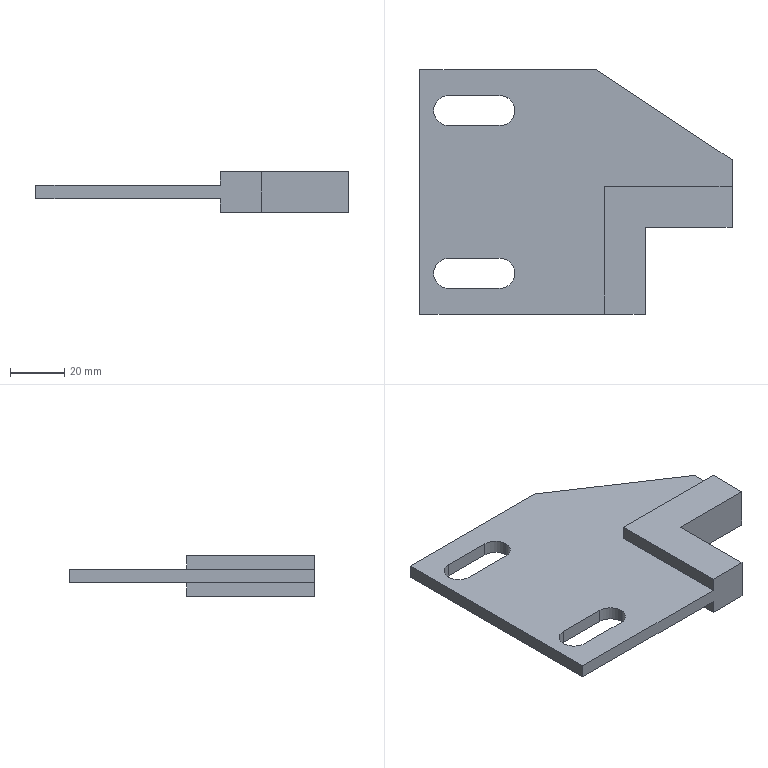Part | SolidWorks | features ICE 2, FlatPattern 1, SMBaseFlange 1, SheetMetal 1 | 1 solid | 25 faces | box 115 x 90 x 15 mm | volume 51294 mm3 | plane 19 | cylinder 6 | commonest cylinder face diameters 11 x6
STEP:
#1=CARTESIAN_POINT('',(35.,-15.,-5.));
#2=VERTEX_POINT('',#1);
#3=CARTESIAN_POINT('',(29.5,-9.5,-5.));
#4=VERTEX_POINT('',#3);
#5=CARTESIAN_POINT('',(29.5,-15.,-5.));
#6=DIRECTION('',(0.,0.,1.));
#7=DIRECTION('',(1.,0.,0.));
#8=AXIS2_PLACEMENT_3D('',#5,#6,#7);
#9=CIRCLE('',#8,5.5);
#10=EDGE_CURVE('',#2,#4,#9,.T.);
#11=ORIENTED_EDGE('',*,*,#10,.F.);
#12=CARTESIAN_POINT('',(35.,-15.,0.));
#13=VERTEX_POINT('',#12);
#14=CARTESIAN_POINT('',(35.,-15.,-5.));
#15=DIRECTION('',(0.,0.,1.));
#16=VECTOR('',#15,1000.);
#17=LINE('',#14,#16);
#18=EDGE_CURVE('',#2,#13,#17,.T.);
#19=ORIENTED_EDGE('',*,*,#18,.T.);
#20=CARTESIAN_POINT('',(29.5,-9.5,0.));
#21=VERTEX_POINT('',#20);
#22=CARTESIAN_POINT('',(29.5,-15.,0.));
#23=DIRECTION('',(0.,0.,1.));
#24=DIRECTION('',(1.,0.,0.));
#25=AXIS2_PLACEMENT_3D('',#22,#23,#24);
#26=CIRCLE('',#25,5.5);
#27=EDGE_CURVE('',#13,#21,#26,.T.);
#28=ORIENTED_EDGE('',*,*,#27,.T.);
#29=CARTESIAN_POINT('',(29.5,-9.5,-5.));
#30=DIRECTION('',(0.,0.,1.));
#31=VECTOR('',#30,1000.);
#32=LINE('',#29,#31);
#33=EDGE_CURVE('',#4,#21,#32,.T.);
#34=ORIENTED_EDGE('',*,*,#33,.F.);
#35=EDGE_LOOP('',(#11,#19,#28,#34));
#36=FACE_OUTER_BOUND('',#35,.T.);
#37=CARTESIAN_POINT('',(29.5,-15.,-5.));
#38=DIRECTION('',(0.,0.,1.));
#39=DIRECTION('',(1.,0.,0.));
#40=AXIS2_PLACEMENT_3D('',#37,#38,#39);
#41=CYLINDRICAL_SURFACE('',#40,5.5);
#42=ADVANCED_FACE('',(#36),#41,.F.);
#43=CARTESIAN_POINT('',(35.,-75.,-5.));
#44=VERTEX_POINT('',#43);
#45=CARTESIAN_POINT('',(29.5,-69.5,-5.));
#46=VERTEX_POINT('',#45);
#47=CARTESIAN_POINT('',(29.5,-75.,-5.));
#48=DIRECTION('',(0.,0.,1.));
#49=DIRECTION('',(-1.,0.,0.));
#50=AXIS2_PLACEMENT_3D('',#47,#48,#49);
#51=CIRCLE('',#50,5.5);
#52=EDGE_CURVE('',#44,#46,#51,.T.);
#53=ORIENTED_EDGE('',*,*,#52,.F.);
#54=CARTESIAN_POINT('',(35.,-75.,0.));
#55=VERTEX_POINT('',#54);
#56=CARTESIAN_POINT('',(35.,-75.,-5.));
#57=DIRECTION('',(0.,0.,1.));
#58=VECTOR('',#57,1000.);
#59=LINE('',#56,#58);
#60=EDGE_CURVE('',#44,#55,#59,.T.);
#61=ORIENTED_EDGE('',*,*,#60,.T.);
#62=CARTESIAN_POINT('',(29.5,-69.5,0.));
#63=VERTEX_POINT('',#62);
#64=CARTESIAN_POINT('',(29.5,-75.,0.));
#65=DIRECTION('',(0.,0.,1.));
#66=DIRECTION('',(-1.,0.,0.));
#67=AXIS2_PLACEMENT_3D('',#64,#65,#66);
#68=CIRCLE('',#67,5.5);
#69=EDGE_CURVE('',#55,#63,#68,.T.);
#70=ORIENTED_EDGE('',*,*,#69,.T.);
#71=CARTESIAN_POINT('',(29.5,-69.5,-5.));
#72=DIRECTION('',(0.,0.,1.));
#73=VECTOR('',#72,1000.);
#74=LINE('',#71,#73);
#75=EDGE_CURVE('',#46,#63,#74,.T.);
#76=ORIENTED_EDGE('',*,*,#75,.F.);
#77=EDGE_LOOP('',(#53,#61,#70,#76));
#78=FACE_OUTER_BOUND('',#77,.T.);
#79=CARTESIAN_POINT('',(29.5,-75.,-5.));
#80=DIRECTION('',(0.,0.,1.));
#81=DIRECTION('',(1.,0.,0.));
#82=AXIS2_PLACEMENT_3D('',#79,#80,#81);
#83=CYLINDRICAL_SURFACE('',#82,5.5);
#84=ADVANCED_FACE('',(#78),#83,.F.);
#85=CARTESIAN_POINT('',(0.,0.,0.));
#86=VERTEX_POINT('',#85);
#87=CARTESIAN_POINT('',(0.,-90.,0.));
#88=VERTEX_POINT('',#87);
#89=CARTESIAN_POINT('',(0.,0.,0.));
#90=DIRECTION('',(0.,-1.,0.));
#91=VECTOR('',#90,1000.);
#92=LINE('',#89,#91);
#93=EDGE_CURVE('',#86,#88,#92,.T.);
#94=ORIENTED_EDGE('',*,*,#93,.F.);
#95=CARTESIAN_POINT('',(0.,0.,-5.));
#96=VERTEX_POINT('',#95);
#97=CARTESIAN_POINT('',(0.,0.,-5.));
#98=DIRECTION('',(0.,0.,1.));
#99=VECTOR('',#98,1000.);
#100=LINE('',#97,#99);
#101=EDGE_CURVE('',#96,#86,#100,.T.);
#102=ORIENTED_EDGE('',*,*,#101,.F.);
#103=CARTESIAN_POINT('',(0.,-90.,-5.));
#104=VERTEX_POINT('',#103);
#105=CARTESIAN_POINT('',(0.,0.,-5.));
#106=DIRECTION('',(0.,-1.,0.));
#107=VECTOR('',#106,1000.);
#108=LINE('',#105,#107);
#109=EDGE_CURVE('',#96,#104,#108,.T.);
#110=ORIENTED_EDGE('',*,*,#109,.T.);
#111=CARTESIAN_POINT('',(0.,-90.,-5.));
#112=DIRECTION('',(0.,0.,1.));
#113=VECTOR('',#112,1000.);
#114=LINE('',#111,#113);
#115=EDGE_CURVE('',#104,#88,#114,.T.);
#116=ORIENTED_EDGE('',*,*,#115,.T.);
#117=EDGE_LOOP('',(#94,#102,#110,#116));
#118=FACE_OUTER_BOUND('',#117,.T.);
#119=CARTESIAN_POINT('',(0.,0.,-5.));
#120=DIRECTION('',(-1.,0.,0.));
#121=DIRECTION('',(0.,-1.,0.));
#122=AXIS2_PLACEMENT_3D('',#119,#120,#121);
#123=PLANE('',#122);
#124=ADVANCED_FACE('',(#118),#123,.T.);
#125=CARTESIAN_POINT('',(65.,0.,0.));
#126=VERTEX_POINT('',#125);
#127=CARTESIAN_POINT('',(0.,0.,0.));
#128=DIRECTION('',(-1.,0.,0.));
#129=VECTOR('',#128,1000.);
#130=LINE('',#127,#129);
#131=EDGE_CURVE('',#126,#86,#130,.T.);
#132=ORIENTED_EDGE('',*,*,#131,.F.);
#133=CARTESIAN_POINT('',(65.,0.,-5.));
#134=VERTEX_POINT('',#133);
#135=CARTESIAN_POINT('',(65.,0.,-5.));
#136=DIRECTION('',(0.,0.,1.));
#137=VECTOR('',#136,1000.);
#138=LINE('',#135,#137);
#139=EDGE_CURVE('',#134,#126,#138,.T.);
#140=ORIENTED_EDGE('',*,*,#139,.F.);
#141=CARTESIAN_POINT('',(0.,0.,-5.));
#142=DIRECTION('',(-1.,0.,0.));
#143=VECTOR('',#142,1000.);
#144=LINE('',#141,#143);
#145=EDGE_CURVE('',#134,#96,#144,.T.);
#146=ORIENTED_EDGE('',*,*,#145,.T.);
#147=ORIENTED_EDGE('',*,*,#101,.T.);
#148=EDGE_LOOP('',(#132,#140,#146,#147));
#149=FACE_OUTER_BOUND('',#148,.T.);
#150=CARTESIAN_POINT('',(0.,0.,-5.));
#151=DIRECTION('',(0.,1.,0.));
#152=DIRECTION('',(0.,0.,1.));
#153=AXIS2_PLACEMENT_3D('',#150,#151,#152);
#154=PLANE('',#153);
#155=ADVANCED_FACE('',(#149),#154,.T.);
#156=CARTESIAN_POINT('',(115.,-33.166,0.));
#157=VERTEX_POINT('',#156);
#158=CARTESIAN_POINT('',(65.,0.,0.));
#159=DIRECTION('',(-0.8333,0.5528,0.));
#160=VECTOR('',#159,1000.);
#161=LINE('',#158,#160);
#162=EDGE_CURVE('',#157,#126,#161,.T.);
#163=ORIENTED_EDGE('',*,*,#162,.F.);
#164=CARTESIAN_POINT('',(115.,-33.166,-5.));
#165=VERTEX_POINT('',#164);
#166=CARTESIAN_POINT('',(115.,-33.166,-5.));
#167=DIRECTION('',(0.,0.,1.));
#168=VECTOR('',#167,1000.);
#169=LINE('',#166,#168);
#170=EDGE_CURVE('',#165,#157,#169,.T.);
#171=ORIENTED_EDGE('',*,*,#170,.F.);
#172=CARTESIAN_POINT('',(65.,0.,-5.));
#173=DIRECTION('',(-0.8333,0.5528,0.));
#174=VECTOR('',#173,1000.);
#175=LINE('',#172,#174);
#176=EDGE_CURVE('',#165,#134,#175,.T.);
#177=ORIENTED_EDGE('',*,*,#176,.T.);
#178=ORIENTED_EDGE('',*,*,#139,.T.);
#179=EDGE_LOOP('',(#163,#171,#177,#178));
#180=FACE_OUTER_BOUND('',#179,.T.);
#181=CARTESIAN_POINT('',(65.,0.,-5.));
#182=DIRECTION('',(0.5528,0.8333,0.));
#183=DIRECTION('',(-0.8333,0.5528,0.));
#184=AXIS2_PLACEMENT_3D('',#181,#182,#183);
#185=PLANE('',#184);
#186=ADVANCED_FACE('',(#180),#185,.T.);
#187=CARTESIAN_POINT('',(115.,-43.,0.));
#188=VERTEX_POINT('',#187);
#189=CARTESIAN_POINT('',(115.,-33.166,0.));
#190=DIRECTION('',(0.,1.,0.));
#191=VECTOR('',#190,1000.);
#192=LINE('',#189,#191);
#193=EDGE_CURVE('',#188,#157,#192,.T.);
#194=ORIENTED_EDGE('',*,*,#193,.F.);
#195=CARTESIAN_POINT('',(115.,-43.,5.));
#196=VERTEX_POINT('',#195);
#197=CARTESIAN_POINT('',(115.,-43.,-10.));
#198=DIRECTION('',(0.,0.,1.));
#199=VECTOR('',#198,1000.);
#200=LINE('',#197,#199);
#201=EDGE_CURVE('',#188,#196,#200,.T.);
#202=ORIENTED_EDGE('',*,*,#201,.T.);
#203=CARTESIAN_POINT('',(115.,-58.,5.));
#204=VERTEX_POINT('',#203);
#205=CARTESIAN_POINT('',(115.,-43.,5.));
#206=DIRECTION('',(0.,1.,0.));
#207=VECTOR('',#206,1000.);
#208=LINE('',#205,#207);
#209=EDGE_CURVE('',#204,#196,#208,.T.);
#210=ORIENTED_EDGE('',*,*,#209,.F.);
#211=CARTESIAN_POINT('',(115.,-58.,-10.));
#212=VERTEX_POINT('',#211);
#213=CARTESIAN_POINT('',(115.,-58.,-10.));
#214=DIRECTION('',(0.,0.,1.));
#215=VECTOR('',#214,1000.);
#216=LINE('',#213,#215);
#217=EDGE_CURVE('',#212,#204,#216,.T.);
#218=ORIENTED_EDGE('',*,*,#217,.F.);
#219=CARTESIAN_POINT('',(115.,-43.,-10.));
#220=VERTEX_POINT('',#219);
#221=CARTESIAN_POINT('',(115.,-43.,-10.));
#222=DIRECTION('',(0.,1.,0.));
#223=VECTOR('',#222,1000.);
#224=LINE('',#221,#223);
#225=EDGE_CURVE('',#212,#220,#224,.T.);
#226=ORIENTED_EDGE('',*,*,#225,.T.);
#227=CARTESIAN_POINT('',(115.,-43.,-5.));
#228=VERTEX_POINT('',#227);
#229=CARTESIAN_POINT('',(115.,-43.,-10.));
#230=DIRECTION('',(0.,0.,1.));
#231=VECTOR('',#230,1000.);
#232=LINE('',#229,#231);
#233=EDGE_CURVE('',#220,#228,#232,.T.);
#234=ORIENTED_EDGE('',*,*,#233,.T.);
#235=CARTESIAN_POINT('',(115.,-33.166,-5.));
#236=DIRECTION('',(0.,1.,0.));
#237=VECTOR('',#236,1000.);
#238=LINE('',#235,#237);
#239=EDGE_CURVE('',#228,#165,#238,.T.);
#240=ORIENTED_EDGE('',*,*,#239,.T.);
#241=ORIENTED_EDGE('',*,*,#170,.T.);
#242=EDGE_LOOP('',(#194,#202,#210,#218,#226,#234,#240,#241));
#243=FACE_OUTER_BOUND('',#242,.T.);
#244=CARTESIAN_POINT('',(115.,-33.166,-5.));
#245=DIRECTION('',(1.,0.,0.));
#246=DIRECTION('',(0.,0.,-1.));
#247=AXIS2_PLACEMENT_3D('',#244,#245,#246);
#248=PLANE('',#247);
#249=ADVANCED_FACE('',(#243),#248,.T.);
#250=CARTESIAN_POINT('',(68.,-90.,0.));
#251=VERTEX_POINT('',#250);
#252=CARTESIAN_POINT('',(0.,-90.,0.));
#253=DIRECTION('',(1.,0.,0.));
#254=VECTOR('',#253,1000.);
#255=LINE('',#252,#254);
#256=EDGE_CURVE('',#88,#251,#255,.T.);
#257=ORIENTED_EDGE('',*,*,#256,.F.);
#258=ORIENTED_EDGE('',*,*,#115,.F.);
#259=CARTESIAN_POINT('',(68.,-90.,-5.));
#260=VERTEX_POINT('',#259);
#261=CARTESIAN_POINT('',(0.,-90.,-5.));
#262=DIRECTION('',(1.,0.,0.));
#263=VECTOR('',#262,1000.);
#264=LINE('',#261,#263);
#265=EDGE_CURVE('',#104,#260,#264,.T.);
#266=ORIENTED_EDGE('',*,*,#265,.T.);
#267=CARTESIAN_POINT('',(68.,-90.,-10.));
#268=VERTEX_POINT('',#267);
#269=CARTESIAN_POINT('',(68.,-90.,-10.));
#270=DIRECTION('',(0.,0.,1.));
#271=VECTOR('',#270,1000.);
#272=LINE('',#269,#271);
#273=EDGE_CURVE('',#268,#260,#272,.T.);
#274=ORIENTED_EDGE('',*,*,#273,.F.);
#275=CARTESIAN_POINT('',(83.,-90.,-10.));
#276=VERTEX_POINT('',#275);
#277=CARTESIAN_POINT('',(68.,-90.,-10.));
#278=DIRECTION('',(1.,0.,0.));
#279=VECTOR('',#278,1000.);
#280=LINE('',#277,#279);
#281=EDGE_CURVE('',#268,#276,#280,.T.);
#282=ORIENTED_EDGE('',*,*,#281,.T.);
#283=CARTESIAN_POINT('',(83.,-90.,5.));
#284=VERTEX_POINT('',#283);
#285=CARTESIAN_POINT('',(83.,-90.,-10.));
#286=DIRECTION('',(0.,0.,1.));
#287=VECTOR('',#286,1000.);
#288=LINE('',#285,#287);
#289=EDGE_CURVE('',#276,#284,#288,.T.);
#290=ORIENTED_EDGE('',*,*,#289,.T.);
#291=CARTESIAN_POINT('',(68.,-90.,5.));
#292=VERTEX_POINT('',#291);
#293=CARTESIAN_POINT('',(68.,-90.,5.));
#294=DIRECTION('',(1.,0.,0.));
#295=VECTOR('',#294,1000.);
#296=LINE('',#293,#295);
#297=EDGE_CURVE('',#292,#284,#296,.T.);
#298=ORIENTED_EDGE('',*,*,#297,.F.);
#299=CARTESIAN_POINT('',(68.,-90.,-10.));
#300=DIRECTION('',(0.,0.,1.));
#301=VECTOR('',#300,1000.);
#302=LINE('',#299,#301);
#303=EDGE_CURVE('',#251,#292,#302,.T.);
#304=ORIENTED_EDGE('',*,*,#303,.F.);
#305=EDGE_LOOP('',(#257,#258,#266,#274,#282,#290,#298,#304));
#306=FACE_OUTER_BOUND('',#305,.T.);
#307=CARTESIAN_POINT('',(0.,-90.,-5.));
#308=DIRECTION('',(0.,-1.,0.));
#309=DIRECTION('',(0.,0.,-1.));
#310=AXIS2_PLACEMENT_3D('',#307,#308,#309);
#311=PLANE('',#310);
#312=ADVANCED_FACE('',(#306),#311,.T.);
#313=CARTESIAN_POINT('',(10.5,-9.5,-5.));
#314=VERTEX_POINT('',#313);
#315=CARTESIAN_POINT('',(10.5,-9.5,-5.));
#316=DIRECTION('',(-1.,0.,0.));
#317=VECTOR('',#316,1000.);
#318=LINE('',#315,#317);
#319=EDGE_CURVE('',#4,#314,#318,.T.);
#320=ORIENTED_EDGE('',*,*,#319,.T.);
#321=CARTESIAN_POINT('',(10.5,-20.5,-5.));
#322=VERTEX_POINT('',#321);
#323=CARTESIAN_POINT('',(10.5,-15.,-5.));
#324=DIRECTION('',(0.,0.,1.));
#325=DIRECTION('',(1.,0.,0.));
#326=AXIS2_PLACEMENT_3D('',#323,#324,#325);
#327=CIRCLE('',#326,5.5);
#328=EDGE_CURVE('',#314,#322,#327,.T.);
#329=ORIENTED_EDGE('',*,*,#328,.T.);
#330=CARTESIAN_POINT('',(29.5,-20.5,-5.));
#331=VERTEX_POINT('',#330);
#332=CARTESIAN_POINT('',(10.5,-20.5,-5.));
#333=DIRECTION('',(1.,0.,0.));
#334=VECTOR('',#333,1000.);
#335=LINE('',#332,#334);
#336=EDGE_CURVE('',#322,#331,#335,.T.);
#337=ORIENTED_EDGE('',*,*,#336,.T.);
#338=CARTESIAN_POINT('',(29.5,-15.,-5.));
#339=DIRECTION('',(0.,0.,1.));
#340=DIRECTION('',(1.,0.,0.));
#341=AXIS2_PLACEMENT_3D('',#338,#339,#340);
#342=CIRCLE('',#341,5.5);
#343=EDGE_CURVE('',#331,#2,#342,.T.);
#344=ORIENTED_EDGE('',*,*,#343,.T.);
#345=ORIENTED_EDGE('',*,*,#10,.T.);
#346=EDGE_LOOP('',(#320,#329,#337,#344,#345));
#347=FACE_BOUND('',#346,.T.);
#348=CARTESIAN_POINT('',(10.5,-69.5,-5.));
#349=VERTEX_POINT('',#348);
#350=CARTESIAN_POINT('',(10.5,-69.5,-5.));
#351=DIRECTION('',(-1.,0.,0.));
#352=VECTOR('',#351,1000.);
#353=LINE('',#350,#352);
#354=EDGE_CURVE('',#46,#349,#353,.T.);
#355=ORIENTED_EDGE('',*,*,#354,.T.);
#356=CARTESIAN_POINT('',(10.5,-80.5,-5.));
#357=VERTEX_POINT('',#356);
#358=CARTESIAN_POINT('',(10.5,-75.,-5.));
#359=DIRECTION('',(0.,0.,1.));
#360=DIRECTION('',(-1.,0.,0.));
#361=AXIS2_PLACEMENT_3D('',#358,#359,#360);
#362=CIRCLE('',#361,5.5);
#363=EDGE_CURVE('',#349,#357,#362,.T.);
#364=ORIENTED_EDGE('',*,*,#363,.T.);
#365=CARTESIAN_POINT('',(29.5,-80.5,-5.));
#366=VERTEX_POINT('',#365);
#367=CARTESIAN_POINT('',(10.5,-80.5,-5.));
#368=DIRECTION('',(1.,0.,0.));
#369=VECTOR('',#368,1000.);
#370=LINE('',#367,#369);
#371=EDGE_CURVE('',#357,#366,#370,.T.);
#372=ORIENTED_EDGE('',*,*,#371,.T.);
#373=CARTESIAN_POINT('',(29.5,-75.,-5.));
#374=DIRECTION('',(0.,0.,1.));
#375=DIRECTION('',(-1.,0.,0.));
#376=AXIS2_PLACEMENT_3D('',#373,#374,#375);
#377=CIRCLE('',#376,5.5);
#378=EDGE_CURVE('',#366,#44,#377,.T.);
#379=ORIENTED_EDGE('',*,*,#378,.T.);
#380=ORIENTED_EDGE('',*,*,#52,.T.);
#381=EDGE_LOOP('',(#355,#364,#372,#379,#380));
#382=FACE_BOUND('',#381,.T.);
#383=ORIENTED_EDGE('',*,*,#109,.F.);
#384=ORIENTED_EDGE('',*,*,#145,.F.);
#385=ORIENTED_EDGE('',*,*,#176,.F.);
#386=ORIENTED_EDGE('',*,*,#239,.F.);
#387=CARTESIAN_POINT('',(68.,-43.,-5.));
#388=VERTEX_POINT('',#387);
#389=CARTESIAN_POINT('',(68.,-43.,-5.));
#390=DIRECTION('',(1.,0.,0.));
#391=VECTOR('',#390,1000.);
#392=LINE('',#389,#391);
#393=EDGE_CURVE('',#388,#228,#392,.T.);
#394=ORIENTED_EDGE('',*,*,#393,.F.);
#395=CARTESIAN_POINT('',(68.,-90.,-5.));
#396=DIRECTION('',(0.,1.,0.));
#397=VECTOR('',#396,1000.);
#398=LINE('',#395,#397);
#399=EDGE_CURVE('',#260,#388,#398,.T.);
#400=ORIENTED_EDGE('',*,*,#399,.F.);
#401=ORIENTED_EDGE('',*,*,#265,.F.);
#402=EDGE_LOOP('',(#383,#384,#385,#386,#394,#400,#401));
#403=FACE_OUTER_BOUND('',#402,.T.);
#404=CARTESIAN_POINT('',(0.,0.,-5.));
#405=DIRECTION('',(0.,0.,1.));
#406=DIRECTION('',(1.,0.,0.));
#407=AXIS2_PLACEMENT_3D('',#404,#405,#406);
#408=PLANE('',#407);
#409=ADVANCED_FACE('',(#347,#382,#403),#408,.F.);
#410=CARTESIAN_POINT('',(10.5,-9.5,0.));
#411=VERTEX_POINT('',#410);
#412=CARTESIAN_POINT('',(10.5,-20.5,0.));
#413=VERTEX_POINT('',#412);
#414=CARTESIAN_POINT('',(10.5,-15.,0.));
#415=DIRECTION('',(0.,0.,1.));
#416=DIRECTION('',(1.,0.,0.));
#417=AXIS2_PLACEMENT_3D('',#414,#415,#416);
#418=CIRCLE('',#417,5.5);
#419=EDGE_CURVE('',#411,#413,#418,.T.);
#420=ORIENTED_EDGE('',*,*,#419,.F.);
#421=CARTESIAN_POINT('',(10.5,-9.5,0.));
#422=DIRECTION('',(-1.,0.,0.));
#423=VECTOR('',#422,1000.);
#424=LINE('',#421,#423);
#425=EDGE_CURVE('',#21,#411,#424,.T.);
#426=ORIENTED_EDGE('',*,*,#425,.F.);
#427=ORIENTED_EDGE('',*,*,#27,.F.);
#428=CARTESIAN_POINT('',(29.5,-20.5,0.));
#429=VERTEX_POINT('',#428);
#430=CARTESIAN_POINT('',(29.5,-15.,0.));
#431=DIRECTION('',(0.,0.,1.));
#432=DIRECTION('',(1.,0.,0.));
#433=AXIS2_PLACEMENT_3D('',#430,#431,#432);
#434=CIRCLE('',#433,5.5);
#435=EDGE_CURVE('',#429,#13,#434,.T.);
#436=ORIENTED_EDGE('',*,*,#435,.F.);
#437=CARTESIAN_POINT('',(10.5,-20.5,0.));
#438=DIRECTION('',(1.,0.,0.));
#439=VECTOR('',#438,1000.);
#440=LINE('',#437,#439);
#441=EDGE_CURVE('',#413,#429,#440,.T.);
#442=ORIENTED_EDGE('',*,*,#441,.F.);
#443=EDGE_LOOP('',(#420,#426,#427,#436,#442));
#444=FACE_BOUND('',#443,.T.);
#445=CARTESIAN_POINT('',(10.5,-69.5,0.));
#446=VERTEX_POINT('',#445);
#447=CARTESIAN_POINT('',(10.5,-80.5,0.));
#448=VERTEX_POINT('',#447);
#449=CARTESIAN_POINT('',(10.5,-75.,0.));
#450=DIRECTION('',(0.,0.,1.));
#451=DIRECTION('',(-1.,0.,0.));
#452=AXIS2_PLACEMENT_3D('',#449,#450,#451);
#453=CIRCLE('',#452,5.5);
#454=EDGE_CURVE('',#446,#448,#453,.T.);
#455=ORIENTED_EDGE('',*,*,#454,.F.);
#456=CARTESIAN_POINT('',(10.5,-69.5,0.));
#457=DIRECTION('',(-1.,0.,0.));
#458=VECTOR('',#457,1000.);
#459=LINE('',#456,#458);
#460=EDGE_CURVE('',#63,#446,#459,.T.);
#461=ORIENTED_EDGE('',*,*,#460,.F.);
#462=ORIENTED_EDGE('',*,*,#69,.F.);
#463=CARTESIAN_POINT('',(29.5,-80.5,0.));
#464=VERTEX_POINT('',#463);
#465=CARTESIAN_POINT('',(29.5,-75.,0.));
#466=DIRECTION('',(0.,0.,1.));
#467=DIRECTION('',(-1.,0.,0.));
#468=AXIS2_PLACEMENT_3D('',#465,#466,#467);
#469=CIRCLE('',#468,5.5);
#470=EDGE_CURVE('',#464,#55,#469,.T.);
#471=ORIENTED_EDGE('',*,*,#470,.F.);
#472=CARTESIAN_POINT('',(10.5,-80.5,0.));
#473=DIRECTION('',(1.,0.,0.));
#474=VECTOR('',#473,1000.);
#475=LINE('',#472,#474);
#476=EDGE_CURVE('',#448,#464,#475,.T.);
#477=ORIENTED_EDGE('',*,*,#476,.F.);
#478=EDGE_LOOP('',(#455,#461,#462,#471,#477));
#479=FACE_BOUND('',#478,.T.);
#480=ORIENTED_EDGE('',*,*,#93,.T.);
#481=ORIENTED_EDGE('',*,*,#256,.T.);
#482=CARTESIAN_POINT('',(68.,-43.,0.));
#483=VERTEX_POINT('',#482);
#484=CARTESIAN_POINT('',(68.,-90.,0.));
#485=DIRECTION('',(0.,1.,0.));
#486=VECTOR('',#485,1000.);
#487=LINE('',#484,#486);
#488=EDGE_CURVE('',#251,#483,#487,.T.);
#489=ORIENTED_EDGE('',*,*,#488,.T.);
#490=CARTESIAN_POINT('',(68.,-43.,0.));
#491=DIRECTION('',(1.,0.,0.));
#492=VECTOR('',#491,1000.);
#493=LINE('',#490,#492);
#494=EDGE_CURVE('',#483,#188,#493,.T.);
#495=ORIENTED_EDGE('',*,*,#494,.T.);
#496=ORIENTED_EDGE('',*,*,#193,.T.);
#497=ORIENTED_EDGE('',*,*,#162,.T.);
#498=ORIENTED_EDGE('',*,*,#131,.T.);
#499=EDGE_LOOP('',(#480,#481,#489,#495,#496,#497,#498));
#500=FACE_OUTER_BOUND('',#499,.T.);
#501=CARTESIAN_POINT('',(0.,0.,0.));
#502=DIRECTION('',(0.,0.,1.));
#503=DIRECTION('',(1.,0.,0.));
#504=AXIS2_PLACEMENT_3D('',#501,#502,#503);
#505=PLANE('',#504);
#506=ADVANCED_FACE('',(#444,#479,#500),#505,.T.);
#507=ORIENTED_EDGE('',*,*,#399,.T.);
#508=CARTESIAN_POINT('',(68.,-43.,-10.));
#509=VERTEX_POINT('',#508);
#510=CARTESIAN_POINT('',(68.,-43.,-10.));
#511=DIRECTION('',(0.,0.,1.));
#512=VECTOR('',#511,1000.);
#513=LINE('',#510,#512);
#514=EDGE_CURVE('',#509,#388,#513,.T.);
#515=ORIENTED_EDGE('',*,*,#514,.F.);
#516=CARTESIAN_POINT('',(68.,-43.,-10.));
#517=DIRECTION('',(0.,-1.,0.));
#518=VECTOR('',#517,1000.);
#519=LINE('',#516,#518);
#520=EDGE_CURVE('',#509,#268,#519,.T.);
#521=ORIENTED_EDGE('',*,*,#520,.T.);
#522=ORIENTED_EDGE('',*,*,#273,.T.);
#523=EDGE_LOOP('',(#507,#515,#521,#522));
#524=FACE_OUTER_BOUND('',#523,.T.);
#525=CARTESIAN_POINT('',(68.,-43.,-10.));
#526=DIRECTION('',(-1.,0.,0.));
#527=DIRECTION('',(0.,-1.,0.));
#528=AXIS2_PLACEMENT_3D('',#525,#526,#527);
#529=PLANE('',#528);
#530=ADVANCED_FACE('',(#524),#529,.T.);
#531=ORIENTED_EDGE('',*,*,#393,.T.);
#532=ORIENTED_EDGE('',*,*,#233,.F.);
#533=CARTESIAN_POINT('',(68.,-43.,-10.));
#534=DIRECTION('',(-1.,0.,0.));
#535=VECTOR('',#534,1000.);
#536=LINE('',#533,#535);
#537=EDGE_CURVE('',#220,#509,#536,.T.);
#538=ORIENTED_EDGE('',*,*,#537,.T.);
#539=ORIENTED_EDGE('',*,*,#514,.T.);
#540=EDGE_LOOP('',(#531,#532,#538,#539));
#541=FACE_OUTER_BOUND('',#540,.T.);
#542=CARTESIAN_POINT('',(68.,-43.,-10.));
#543=DIRECTION('',(0.,1.,0.));
#544=DIRECTION('',(0.,0.,1.));
#545=AXIS2_PLACEMENT_3D('',#542,#543,#544);
#546=PLANE('',#545);
#547=ADVANCED_FACE('',(#541),#546,.T.);
#548=CARTESIAN_POINT('',(68.,-43.,5.));
#549=VERTEX_POINT('',#548);
#550=CARTESIAN_POINT('',(68.,-43.,-10.));
#551=DIRECTION('',(0.,0.,1.));
#552=VECTOR('',#551,1000.);
#553=LINE('',#550,#552);
#554=EDGE_CURVE('',#483,#549,#553,.T.);
#555=ORIENTED_EDGE('',*,*,#554,.F.);
#556=ORIENTED_EDGE('',*,*,#488,.F.);
#557=ORIENTED_EDGE('',*,*,#303,.T.);
#558=CARTESIAN_POINT('',(68.,-43.,5.));
#559=DIRECTION('',(0.,-1.,0.));
#560=VECTOR('',#559,1000.);
#561=LINE('',#558,#560);
#562=EDGE_CURVE('',#549,#292,#561,.T.);
#563=ORIENTED_EDGE('',*,*,#562,.F.);
#564=EDGE_LOOP('',(#555,#556,#557,#563));
#565=FACE_OUTER_BOUND('',#564,.T.);
#566=CARTESIAN_POINT('',(68.,-43.,-10.));
#567=DIRECTION('',(-1.,0.,0.));
#568=DIRECTION('',(0.,-1.,0.));
#569=AXIS2_PLACEMENT_3D('',#566,#567,#568);
#570=PLANE('',#569);
#571=ADVANCED_FACE('',(#565),#570,.T.);
#572=ORIENTED_EDGE('',*,*,#201,.F.);
#573=ORIENTED_EDGE('',*,*,#494,.F.);
#574=ORIENTED_EDGE('',*,*,#554,.T.);
#575=CARTESIAN_POINT('',(68.,-43.,5.));
#576=DIRECTION('',(-1.,0.,0.));
#577=VECTOR('',#576,1000.);
#578=LINE('',#575,#577);
#579=EDGE_CURVE('',#196,#549,#578,.T.);
#580=ORIENTED_EDGE('',*,*,#579,.F.);
#581=EDGE_LOOP('',(#572,#573,#574,#580));
#582=FACE_OUTER_BOUND('',#581,.T.);
#583=CARTESIAN_POINT('',(68.,-43.,-10.));
#584=DIRECTION('',(0.,1.,0.));
#585=DIRECTION('',(0.,0.,1.));
#586=AXIS2_PLACEMENT_3D('',#583,#584,#585);
#587=PLANE('',#586);
#588=ADVANCED_FACE('',(#582),#587,.T.);
#589=ORIENTED_EDGE('',*,*,#217,.T.);
#590=CARTESIAN_POINT('',(83.,-58.,5.));
#591=VERTEX_POINT('',#590);
#592=CARTESIAN_POINT('',(115.,-58.,5.));
#593=DIRECTION('',(1.,0.,0.));
#594=VECTOR('',#593,1000.);
#595=LINE('',#592,#594);
#596=EDGE_CURVE('',#591,#204,#595,.T.);
#597=ORIENTED_EDGE('',*,*,#596,.F.);
#598=CARTESIAN_POINT('',(83.,-58.,-10.));
#599=VERTEX_POINT('',#598);
#600=CARTESIAN_POINT('',(83.,-58.,-10.));
#601=DIRECTION('',(0.,0.,1.));
#602=VECTOR('',#601,1000.);
#603=LINE('',#600,#602);
#604=EDGE_CURVE('',#599,#591,#603,.T.);
#605=ORIENTED_EDGE('',*,*,#604,.F.);
#606=CARTESIAN_POINT('',(115.,-58.,-10.));
#607=DIRECTION('',(1.,0.,0.));
#608=VECTOR('',#607,1000.);
#609=LINE('',#606,#608);
#610=EDGE_CURVE('',#599,#212,#609,.T.);
#611=ORIENTED_EDGE('',*,*,#610,.T.);
#612=EDGE_LOOP('',(#589,#597,#605,#611));
#613=FACE_OUTER_BOUND('',#612,.T.);
#614=CARTESIAN_POINT('',(115.,-58.,-10.));
#615=DIRECTION('',(0.,-1.,0.));
#616=DIRECTION('',(1.,0.,0.));
#617=AXIS2_PLACEMENT_3D('',#614,#615,#616);
#618=PLANE('',#617);
#619=ADVANCED_FACE('',(#613),#618,.T.);
#620=ORIENTED_EDGE('',*,*,#604,.T.);
#621=CARTESIAN_POINT('',(83.,-90.,5.));
#622=DIRECTION('',(0.,1.,0.));
#623=VECTOR('',#622,1000.);
#624=LINE('',#621,#623);
#625=EDGE_CURVE('',#284,#591,#624,.T.);
#626=ORIENTED_EDGE('',*,*,#625,.F.);
#627=ORIENTED_EDGE('',*,*,#289,.F.);
#628=CARTESIAN_POINT('',(83.,-90.,-10.));
#629=DIRECTION('',(0.,1.,0.));
#630=VECTOR('',#629,1000.);
#631=LINE('',#628,#630);
#632=EDGE_CURVE('',#276,#599,#631,.T.);
#633=ORIENTED_EDGE('',*,*,#632,.T.);
#634=EDGE_LOOP('',(#620,#626,#627,#633));
#635=FACE_OUTER_BOUND('',#634,.T.);
#636=CARTESIAN_POINT('',(83.,-90.,-10.));
#637=DIRECTION('',(1.,0.,0.));
#638=DIRECTION('',(0.,0.,-1.));
#639=AXIS2_PLACEMENT_3D('',#636,#637,#638);
#640=PLANE('',#639);
#641=ADVANCED_FACE('',(#635),#640,.T.);
#642=ORIENTED_EDGE('',*,*,#520,.F.);
#643=ORIENTED_EDGE('',*,*,#537,.F.);
#644=ORIENTED_EDGE('',*,*,#225,.F.);
#645=ORIENTED_EDGE('',*,*,#610,.F.);
#646=ORIENTED_EDGE('',*,*,#632,.F.);
#647=ORIENTED_EDGE('',*,*,#281,.F.);
#648=EDGE_LOOP('',(#642,#643,#644,#645,#646,#647));
#649=FACE_OUTER_BOUND('',#648,.T.);
#650=CARTESIAN_POINT('',(0.,0.,-10.));
#651=DIRECTION('',(0.,0.,1.));
#652=DIRECTION('',(1.,0.,0.));
#653=AXIS2_PLACEMENT_3D('',#650,#651,#652);
#654=PLANE('',#653);
#655=ADVANCED_FACE('',(#649),#654,.F.);
#656=ORIENTED_EDGE('',*,*,#562,.T.);
#657=ORIENTED_EDGE('',*,*,#297,.T.);
#658=ORIENTED_EDGE('',*,*,#625,.T.);
#659=ORIENTED_EDGE('',*,*,#596,.T.);
#660=ORIENTED_EDGE('',*,*,#209,.T.);
#661=ORIENTED_EDGE('',*,*,#579,.T.);
#662=EDGE_LOOP('',(#656,#657,#658,#659,#660,#661));
#663=FACE_OUTER_BOUND('',#662,.T.);
#664=CARTESIAN_POINT('',(0.,0.,5.));
#665=DIRECTION('',(0.,0.,1.));
#666=DIRECTION('',(1.,0.,0.));
#667=AXIS2_PLACEMENT_3D('',#664,#665,#666);
#668=PLANE('',#667);
#669=ADVANCED_FACE('',(#663),#668,.T.);
#670=ORIENTED_EDGE('',*,*,#454,.T.);
#671=CARTESIAN_POINT('',(10.5,-80.5,-5.));
#672=DIRECTION('',(0.,0.,1.));
#673=VECTOR('',#672,1000.);
#674=LINE('',#671,#673);
#675=EDGE_CURVE('',#357,#448,#674,.T.);
#676=ORIENTED_EDGE('',*,*,#675,.F.);
#677=ORIENTED_EDGE('',*,*,#363,.F.);
#678=CARTESIAN_POINT('',(10.5,-69.5,-5.));
#679=DIRECTION('',(0.,0.,1.));
#680=VECTOR('',#679,1000.);
#681=LINE('',#678,#680);
#682=EDGE_CURVE('',#349,#446,#681,.T.);
#683=ORIENTED_EDGE('',*,*,#682,.T.);
#684=EDGE_LOOP('',(#670,#676,#677,#683));
#685=FACE_OUTER_BOUND('',#684,.T.);
#686=CARTESIAN_POINT('',(10.5,-75.,-5.));
#687=DIRECTION('',(0.,0.,1.));
#688=DIRECTION('',(1.,0.,0.));
#689=AXIS2_PLACEMENT_3D('',#686,#687,#688);
#690=CYLINDRICAL_SURFACE('',#689,5.5);
#691=ADVANCED_FACE('',(#685),#690,.F.);
#692=ORIENTED_EDGE('',*,*,#460,.T.);
#693=ORIENTED_EDGE('',*,*,#682,.F.);
#694=ORIENTED_EDGE('',*,*,#354,.F.);
#695=ORIENTED_EDGE('',*,*,#75,.T.);
#696=EDGE_LOOP('',(#692,#693,#694,#695));
#697=FACE_OUTER_BOUND('',#696,.T.);
#698=CARTESIAN_POINT('',(10.5,-69.5,-5.));
#699=DIRECTION('',(0.,1.,0.));
#700=DIRECTION('',(0.,0.,1.));
#701=AXIS2_PLACEMENT_3D('',#698,#699,#700);
#702=PLANE('',#701);
#703=ADVANCED_FACE('',(#697),#702,.F.);
#704=ORIENTED_EDGE('',*,*,#60,.F.);
#705=ORIENTED_EDGE('',*,*,#378,.F.);
#706=CARTESIAN_POINT('',(29.5,-80.5,-5.));
#707=DIRECTION('',(0.,0.,1.));
#708=VECTOR('',#707,1000.);
#709=LINE('',#706,#708);
#710=EDGE_CURVE('',#366,#464,#709,.T.);
#711=ORIENTED_EDGE('',*,*,#710,.T.);
#712=ORIENTED_EDGE('',*,*,#470,.T.);
#713=EDGE_LOOP('',(#704,#705,#711,#712));
#714=FACE_OUTER_BOUND('',#713,.T.);
#715=CARTESIAN_POINT('',(29.5,-75.,-5.));
#716=DIRECTION('',(0.,0.,1.));
#717=DIRECTION('',(1.,0.,0.));
#718=AXIS2_PLACEMENT_3D('',#715,#716,#717);
#719=CYLINDRICAL_SURFACE('',#718,5.5);
#720=ADVANCED_FACE('',(#714),#719,.F.);
#721=ORIENTED_EDGE('',*,*,#476,.T.);
#722=ORIENTED_EDGE('',*,*,#710,.F.);
#723=ORIENTED_EDGE('',*,*,#371,.F.);
#724=ORIENTED_EDGE('',*,*,#675,.T.);
#725=EDGE_LOOP('',(#721,#722,#723,#724));
#726=FACE_OUTER_BOUND('',#725,.T.);
#727=CARTESIAN_POINT('',(10.5,-80.5,-5.));
#728=DIRECTION('',(0.,-1.,0.));
#729=DIRECTION('',(0.,0.,-1.));
#730=AXIS2_PLACEMENT_3D('',#727,#728,#729);
#731=PLANE('',#730);
#732=ADVANCED_FACE('',(#726),#731,.F.);
#733=ORIENTED_EDGE('',*,*,#419,.T.);
#734=CARTESIAN_POINT('',(10.5,-20.5,-5.));
#735=DIRECTION('',(0.,0.,1.));
#736=VECTOR('',#735,1000.);
#737=LINE('',#734,#736);
#738=EDGE_CURVE('',#322,#413,#737,.T.);
#739=ORIENTED_EDGE('',*,*,#738,.F.);
#740=ORIENTED_EDGE('',*,*,#328,.F.);
#741=CARTESIAN_POINT('',(10.5,-9.5,-5.));
#742=DIRECTION('',(0.,0.,1.));
#743=VECTOR('',#742,1000.);
#744=LINE('',#741,#743);
#745=EDGE_CURVE('',#314,#411,#744,.T.);
#746=ORIENTED_EDGE('',*,*,#745,.T.);
#747=EDGE_LOOP('',(#733,#739,#740,#746));
#748=FACE_OUTER_BOUND('',#747,.T.);
#749=CARTESIAN_POINT('',(10.5,-15.,-5.));
#750=DIRECTION('',(0.,0.,1.));
#751=DIRECTION('',(1.,0.,0.));
#752=AXIS2_PLACEMENT_3D('',#749,#750,#751);
#753=CYLINDRICAL_SURFACE('',#752,5.5);
#754=ADVANCED_FACE('',(#748),#753,.F.);
#755=ORIENTED_EDGE('',*,*,#425,.T.);
#756=ORIENTED_EDGE('',*,*,#745,.F.);
#757=ORIENTED_EDGE('',*,*,#319,.F.);
#758=ORIENTED_EDGE('',*,*,#33,.T.);
#759=EDGE_LOOP('',(#755,#756,#757,#758));
#760=FACE_OUTER_BOUND('',#759,.T.);
#761=CARTESIAN_POINT('',(10.5,-9.5,-5.));
#762=DIRECTION('',(0.,1.,0.));
#763=DIRECTION('',(-1.,0.,0.));
#764=AXIS2_PLACEMENT_3D('',#761,#762,#763);
#765=PLANE('',#764);
#766=ADVANCED_FACE('',(#760),#765,.F.);
#767=ORIENTED_EDGE('',*,*,#18,.F.);
#768=ORIENTED_EDGE('',*,*,#343,.F.);
#769=CARTESIAN_POINT('',(29.5,-20.5,-5.));
#770=DIRECTION('',(0.,0.,1.));
#771=VECTOR('',#770,1000.);
#772=LINE('',#769,#771);
#773=EDGE_CURVE('',#331,#429,#772,.T.);
#774=ORIENTED_EDGE('',*,*,#773,.T.);
#775=ORIENTED_EDGE('',*,*,#435,.T.);
#776=EDGE_LOOP('',(#767,#768,#774,#775));
#777=FACE_OUTER_BOUND('',#776,.T.);
#778=CARTESIAN_POINT('',(29.5,-15.,-5.));
#779=DIRECTION('',(0.,0.,1.));
#780=DIRECTION('',(1.,0.,0.));
#781=AXIS2_PLACEMENT_3D('',#778,#779,#780);
#782=CYLINDRICAL_SURFACE('',#781,5.5);
#783=ADVANCED_FACE('',(#777),#782,.F.);
#784=ORIENTED_EDGE('',*,*,#441,.T.);
#785=ORIENTED_EDGE('',*,*,#773,.F.);
#786=ORIENTED_EDGE('',*,*,#336,.F.);
#787=ORIENTED_EDGE('',*,*,#738,.T.);
#788=EDGE_LOOP('',(#784,#785,#786,#787));
#789=FACE_OUTER_BOUND('',#788,.T.);
#790=CARTESIAN_POINT('',(10.5,-20.5,-5.));
#791=DIRECTION('',(0.,-1.,0.));
#792=DIRECTION('',(1.,0.,0.));
#793=AXIS2_PLACEMENT_3D('',#790,#791,#792);
#794=PLANE('',#793);
#795=ADVANCED_FACE('',(#789),#794,.F.);
#796=CLOSED_SHELL('',(#42,#84,#124,#155,#186,#249,#312,#409,#506,#530,#547,#571,#588,#619,#641,#655,#669,#691,#703,#720,#732,#754,#766,#783,#795));
#797=MANIFOLD_SOLID_BREP('',#796);
#798=CARTESIAN_POINT('',(0.,0.,0.));
#799=DIRECTION('',(0.,0.,1.));
#800=DIRECTION('',(1.,0.,0.));
#801=AXIS2_PLACEMENT_3D('',#798,#799,#800);
#802=(LENGTH_UNIT()NAMED_UNIT(*)SI_UNIT(.MILLI.,.METRE.));
#803=UNCERTAINTY_MEASURE_WITH_UNIT(LENGTH_MEASURE(0.00001),#802,'','');
#804=(NAMED_UNIT(*)PLANE_ANGLE_UNIT()SI_UNIT($,.RADIAN.));
#805=(NAMED_UNIT(*)SI_UNIT($,.STERADIAN.)SOLID_ANGLE_UNIT());
#806=(GEOMETRIC_REPRESENTATION_CONTEXT(3)GLOBAL_UNCERTAINTY_ASSIGNED_CONTEXT((#803))GLOBAL_UNIT_ASSIGNED_CONTEXT((#802,#804,#805))REPRESENTATION_CONTEXT('',''));
#807=ADVANCED_BREP_SHAPE_REPRESENTATION('',(#797,#801),#806);